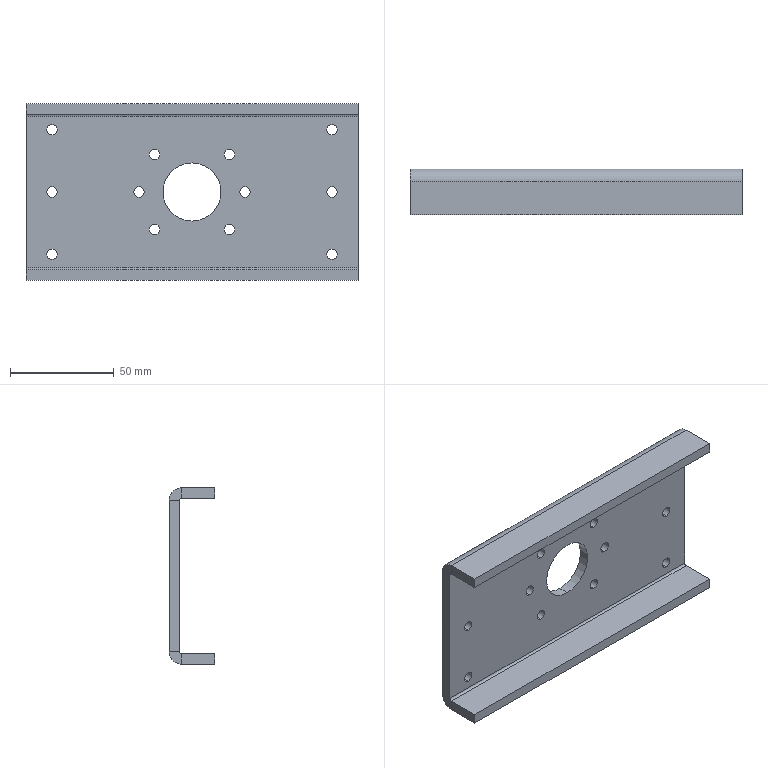Part | SolidWorks | features HoleWzd 2, CirPattern 1, EdgeFlange 1, FlatPattern 1, SMBaseFlange 1, SheetMetal 1 | 1 solid | 48 faces | box 160 x 22 x 85 mm | volume 88540 mm3 | cylinder 30 | plane 18 | commonest cylinder face diameters 5 x24 2 x2 12 x2 28 x2
STEP:
#1=CARTESIAN_POINT('',(18.031,-5.,-20.531));
#2=VERTEX_POINT('',#1);
#3=CARTESIAN_POINT('',(18.031,-5.,-15.531));
#4=VERTEX_POINT('',#3);
#5=CARTESIAN_POINT('',(18.031,-5.,-18.031));
#6=DIRECTION('',(0.,1.,0.));
#7=DIRECTION('',(0.,0.,1.));
#8=AXIS2_PLACEMENT_3D('',#5,#6,#7);
#9=CIRCLE('',#8,2.5);
#10=EDGE_CURVE('',#2,#4,#9,.T.);
#11=ORIENTED_EDGE('',*,*,#10,.F.);
#12=CARTESIAN_POINT('',(18.031,0.,-20.531));
#13=VERTEX_POINT('',#12);
#14=CARTESIAN_POINT('',(18.031,0.,-20.531));
#15=DIRECTION('',(0.,1.,0.));
#16=VECTOR('',#15,1000.);
#17=LINE('',#14,#16);
#18=EDGE_CURVE('',#2,#13,#17,.T.);
#19=ORIENTED_EDGE('',*,*,#18,.T.);
#20=CARTESIAN_POINT('',(18.031,0.,-15.531));
#21=VERTEX_POINT('',#20);
#22=CARTESIAN_POINT('',(18.031,0.,-18.031));
#23=DIRECTION('',(0.,1.,0.));
#24=DIRECTION('',(0.,0.,1.));
#25=AXIS2_PLACEMENT_3D('',#22,#23,#24);
#26=CIRCLE('',#25,2.5);
#27=EDGE_CURVE('',#13,#21,#26,.T.);
#28=ORIENTED_EDGE('',*,*,#27,.T.);
#29=CARTESIAN_POINT('',(18.031,0.,-15.531));
#30=DIRECTION('',(0.,1.,0.));
#31=VECTOR('',#30,1000.);
#32=LINE('',#29,#31);
#33=EDGE_CURVE('',#4,#21,#32,.T.);
#34=ORIENTED_EDGE('',*,*,#33,.F.);
#35=EDGE_LOOP('',(#11,#19,#28,#34));
#36=FACE_OUTER_BOUND('',#35,.T.);
#37=CARTESIAN_POINT('',(18.031,0.,-18.031));
#38=DIRECTION('',(0.,1.,0.));
#39=DIRECTION('',(0.,0.,1.));
#40=AXIS2_PLACEMENT_3D('',#37,#38,#39);
#41=CYLINDRICAL_SURFACE('',#40,2.5);
#42=ADVANCED_FACE('',(#36),#41,.F.);
#43=CARTESIAN_POINT('',(25.5,-5.,-2.5));
#44=VERTEX_POINT('',#43);
#45=CARTESIAN_POINT('',(25.5,-5.,2.5));
#46=VERTEX_POINT('',#45);
#47=CARTESIAN_POINT('',(25.5,-5.,0.));
#48=DIRECTION('',(0.,1.,0.));
#49=DIRECTION('',(0.,0.,1.));
#50=AXIS2_PLACEMENT_3D('',#47,#48,#49);
#51=CIRCLE('',#50,2.5);
#52=EDGE_CURVE('',#44,#46,#51,.T.);
#53=ORIENTED_EDGE('',*,*,#52,.F.);
#54=CARTESIAN_POINT('',(25.5,0.,-2.5));
#55=VERTEX_POINT('',#54);
#56=CARTESIAN_POINT('',(25.5,0.,-2.5));
#57=DIRECTION('',(0.,1.,0.));
#58=VECTOR('',#57,1000.);
#59=LINE('',#56,#58);
#60=EDGE_CURVE('',#44,#55,#59,.T.);
#61=ORIENTED_EDGE('',*,*,#60,.T.);
#62=CARTESIAN_POINT('',(25.5,0.,2.5));
#63=VERTEX_POINT('',#62);
#64=CARTESIAN_POINT('',(25.5,0.,0.));
#65=DIRECTION('',(0.,1.,0.));
#66=DIRECTION('',(0.,0.,1.));
#67=AXIS2_PLACEMENT_3D('',#64,#65,#66);
#68=CIRCLE('',#67,2.5);
#69=EDGE_CURVE('',#55,#63,#68,.T.);
#70=ORIENTED_EDGE('',*,*,#69,.T.);
#71=CARTESIAN_POINT('',(25.5,0.,2.5));
#72=DIRECTION('',(0.,1.,0.));
#73=VECTOR('',#72,1000.);
#74=LINE('',#71,#73);
#75=EDGE_CURVE('',#46,#63,#74,.T.);
#76=ORIENTED_EDGE('',*,*,#75,.F.);
#77=EDGE_LOOP('',(#53,#61,#70,#76));
#78=FACE_OUTER_BOUND('',#77,.T.);
#79=CARTESIAN_POINT('',(25.5,0.,0.));
#80=DIRECTION('',(0.,1.,0.));
#81=DIRECTION('',(0.,0.,1.));
#82=AXIS2_PLACEMENT_3D('',#79,#80,#81);
#83=CYLINDRICAL_SURFACE('',#82,2.5);
#84=ADVANCED_FACE('',(#78),#83,.F.);
#85=CARTESIAN_POINT('',(18.031,-5.,15.531));
#86=VERTEX_POINT('',#85);
#87=CARTESIAN_POINT('',(18.031,-5.,20.531));
#88=VERTEX_POINT('',#87);
#89=CARTESIAN_POINT('',(18.031,-5.,18.031));
#90=DIRECTION('',(0.,1.,0.));
#91=DIRECTION('',(0.,0.,1.));
#92=AXIS2_PLACEMENT_3D('',#89,#90,#91);
#93=CIRCLE('',#92,2.5);
#94=EDGE_CURVE('',#86,#88,#93,.T.);
#95=ORIENTED_EDGE('',*,*,#94,.F.);
#96=CARTESIAN_POINT('',(18.031,0.,15.531));
#97=VERTEX_POINT('',#96);
#98=CARTESIAN_POINT('',(18.031,0.,15.531));
#99=DIRECTION('',(0.,1.,0.));
#100=VECTOR('',#99,1000.);
#101=LINE('',#98,#100);
#102=EDGE_CURVE('',#86,#97,#101,.T.);
#103=ORIENTED_EDGE('',*,*,#102,.T.);
#104=CARTESIAN_POINT('',(18.031,0.,20.531));
#105=VERTEX_POINT('',#104);
#106=CARTESIAN_POINT('',(18.031,0.,18.031));
#107=DIRECTION('',(0.,1.,0.));
#108=DIRECTION('',(0.,0.,1.));
#109=AXIS2_PLACEMENT_3D('',#106,#107,#108);
#110=CIRCLE('',#109,2.5);
#111=EDGE_CURVE('',#97,#105,#110,.T.);
#112=ORIENTED_EDGE('',*,*,#111,.T.);
#113=CARTESIAN_POINT('',(18.031,0.,20.531));
#114=DIRECTION('',(0.,1.,0.));
#115=VECTOR('',#114,1000.);
#116=LINE('',#113,#115);
#117=EDGE_CURVE('',#88,#105,#116,.T.);
#118=ORIENTED_EDGE('',*,*,#117,.F.);
#119=EDGE_LOOP('',(#95,#103,#112,#118));
#120=FACE_OUTER_BOUND('',#119,.T.);
#121=CARTESIAN_POINT('',(18.031,0.,18.031));
#122=DIRECTION('',(0.,1.,0.));
#123=DIRECTION('',(0.,0.,1.));
#124=AXIS2_PLACEMENT_3D('',#121,#122,#123);
#125=CYLINDRICAL_SURFACE('',#124,2.5);
#126=ADVANCED_FACE('',(#120),#125,.F.);
#127=CARTESIAN_POINT('',(-18.031,-5.,15.531));
#128=VERTEX_POINT('',#127);
#129=CARTESIAN_POINT('',(-18.031,-5.,20.531));
#130=VERTEX_POINT('',#129);
#131=CARTESIAN_POINT('',(-18.031,-5.,18.031));
#132=DIRECTION('',(0.,1.,0.));
#133=DIRECTION('',(0.,0.,1.));
#134=AXIS2_PLACEMENT_3D('',#131,#132,#133);
#135=CIRCLE('',#134,2.5);
#136=EDGE_CURVE('',#128,#130,#135,.T.);
#137=ORIENTED_EDGE('',*,*,#136,.F.);
#138=CARTESIAN_POINT('',(-18.031,0.,15.531));
#139=VERTEX_POINT('',#138);
#140=CARTESIAN_POINT('',(-18.031,0.,15.531));
#141=DIRECTION('',(0.,1.,0.));
#142=VECTOR('',#141,1000.);
#143=LINE('',#140,#142);
#144=EDGE_CURVE('',#128,#139,#143,.T.);
#145=ORIENTED_EDGE('',*,*,#144,.T.);
#146=CARTESIAN_POINT('',(-18.031,0.,20.531));
#147=VERTEX_POINT('',#146);
#148=CARTESIAN_POINT('',(-18.031,0.,18.031));
#149=DIRECTION('',(0.,1.,0.));
#150=DIRECTION('',(0.,0.,1.));
#151=AXIS2_PLACEMENT_3D('',#148,#149,#150);
#152=CIRCLE('',#151,2.5);
#153=EDGE_CURVE('',#139,#147,#152,.T.);
#154=ORIENTED_EDGE('',*,*,#153,.T.);
#155=CARTESIAN_POINT('',(-18.031,0.,20.531));
#156=DIRECTION('',(0.,1.,0.));
#157=VECTOR('',#156,1000.);
#158=LINE('',#155,#157);
#159=EDGE_CURVE('',#130,#147,#158,.T.);
#160=ORIENTED_EDGE('',*,*,#159,.F.);
#161=EDGE_LOOP('',(#137,#145,#154,#160));
#162=FACE_OUTER_BOUND('',#161,.T.);
#163=CARTESIAN_POINT('',(-18.031,0.,18.031));
#164=DIRECTION('',(0.,1.,0.));
#165=DIRECTION('',(0.,0.,1.));
#166=AXIS2_PLACEMENT_3D('',#163,#164,#165);
#167=CYLINDRICAL_SURFACE('',#166,2.5);
#168=ADVANCED_FACE('',(#162),#167,.F.);
#169=CARTESIAN_POINT('',(-25.5,-5.,-2.5));
#170=VERTEX_POINT('',#169);
#171=CARTESIAN_POINT('',(-25.5,-5.,2.5));
#172=VERTEX_POINT('',#171);
#173=CARTESIAN_POINT('',(-25.5,-5.,0.));
#174=DIRECTION('',(0.,1.,0.));
#175=DIRECTION('',(0.,0.,1.));
#176=AXIS2_PLACEMENT_3D('',#173,#174,#175);
#177=CIRCLE('',#176,2.5);
#178=EDGE_CURVE('',#170,#172,#177,.T.);
#179=ORIENTED_EDGE('',*,*,#178,.F.);
#180=CARTESIAN_POINT('',(-25.5,0.,-2.5));
#181=VERTEX_POINT('',#180);
#182=CARTESIAN_POINT('',(-25.5,0.,-2.5));
#183=DIRECTION('',(0.,1.,0.));
#184=VECTOR('',#183,1000.);
#185=LINE('',#182,#184);
#186=EDGE_CURVE('',#170,#181,#185,.T.);
#187=ORIENTED_EDGE('',*,*,#186,.T.);
#188=CARTESIAN_POINT('',(-25.5,0.,2.5));
#189=VERTEX_POINT('',#188);
#190=CARTESIAN_POINT('',(-25.5,0.,0.));
#191=DIRECTION('',(0.,1.,0.));
#192=DIRECTION('',(0.,0.,1.));
#193=AXIS2_PLACEMENT_3D('',#190,#191,#192);
#194=CIRCLE('',#193,2.5);
#195=EDGE_CURVE('',#181,#189,#194,.T.);
#196=ORIENTED_EDGE('',*,*,#195,.T.);
#197=CARTESIAN_POINT('',(-25.5,0.,2.5));
#198=DIRECTION('',(0.,1.,0.));
#199=VECTOR('',#198,1000.);
#200=LINE('',#197,#199);
#201=EDGE_CURVE('',#172,#189,#200,.T.);
#202=ORIENTED_EDGE('',*,*,#201,.F.);
#203=EDGE_LOOP('',(#179,#187,#196,#202));
#204=FACE_OUTER_BOUND('',#203,.T.);
#205=CARTESIAN_POINT('',(-25.5,0.,0.));
#206=DIRECTION('',(0.,1.,0.));
#207=DIRECTION('',(0.,0.,1.));
#208=AXIS2_PLACEMENT_3D('',#205,#206,#207);
#209=CYLINDRICAL_SURFACE('',#208,2.5);
#210=ADVANCED_FACE('',(#204),#209,.F.);
#211=CARTESIAN_POINT('',(-18.031,-5.,-20.531));
#212=VERTEX_POINT('',#211);
#213=CARTESIAN_POINT('',(-18.031,-5.,-15.531));
#214=VERTEX_POINT('',#213);
#215=CARTESIAN_POINT('',(-18.031,-5.,-18.031));
#216=DIRECTION('',(0.,1.,0.));
#217=DIRECTION('',(0.,0.,1.));
#218=AXIS2_PLACEMENT_3D('',#215,#216,#217);
#219=CIRCLE('',#218,2.5);
#220=EDGE_CURVE('',#212,#214,#219,.T.);
#221=ORIENTED_EDGE('',*,*,#220,.F.);
#222=CARTESIAN_POINT('',(-18.031,0.,-20.531));
#223=VERTEX_POINT('',#222);
#224=CARTESIAN_POINT('',(-18.031,0.,-20.531));
#225=DIRECTION('',(0.,1.,0.));
#226=VECTOR('',#225,1000.);
#227=LINE('',#224,#226);
#228=EDGE_CURVE('',#212,#223,#227,.T.);
#229=ORIENTED_EDGE('',*,*,#228,.T.);
#230=CARTESIAN_POINT('',(-18.031,0.,-15.531));
#231=VERTEX_POINT('',#230);
#232=CARTESIAN_POINT('',(-18.031,0.,-18.031));
#233=DIRECTION('',(0.,1.,0.));
#234=DIRECTION('',(0.,0.,1.));
#235=AXIS2_PLACEMENT_3D('',#232,#233,#234);
#236=CIRCLE('',#235,2.5);
#237=EDGE_CURVE('',#223,#231,#236,.T.);
#238=ORIENTED_EDGE('',*,*,#237,.T.);
#239=CARTESIAN_POINT('',(-18.031,0.,-15.531));
#240=DIRECTION('',(0.,1.,0.));
#241=VECTOR('',#240,1000.);
#242=LINE('',#239,#241);
#243=EDGE_CURVE('',#214,#231,#242,.T.);
#244=ORIENTED_EDGE('',*,*,#243,.F.);
#245=EDGE_LOOP('',(#221,#229,#238,#244));
#246=FACE_OUTER_BOUND('',#245,.T.);
#247=CARTESIAN_POINT('',(-18.031,0.,-18.031));
#248=DIRECTION('',(0.,1.,0.));
#249=DIRECTION('',(0.,0.,1.));
#250=AXIS2_PLACEMENT_3D('',#247,#248,#249);
#251=CYLINDRICAL_SURFACE('',#250,2.5);
#252=ADVANCED_FACE('',(#246),#251,.F.);
#253=CARTESIAN_POINT('',(-67.5,-5.,-2.5));
#254=VERTEX_POINT('',#253);
#255=CARTESIAN_POINT('',(-67.5,-5.,2.5));
#256=VERTEX_POINT('',#255);
#257=CARTESIAN_POINT('',(-67.5,-5.,0.));
#258=DIRECTION('',(0.,1.,0.));
#259=DIRECTION('',(0.,0.,1.));
#260=AXIS2_PLACEMENT_3D('',#257,#258,#259);
#261=CIRCLE('',#260,2.5);
#262=EDGE_CURVE('',#254,#256,#261,.T.);
#263=ORIENTED_EDGE('',*,*,#262,.F.);
#264=CARTESIAN_POINT('',(-67.5,0.,-2.5));
#265=VERTEX_POINT('',#264);
#266=CARTESIAN_POINT('',(-67.5,0.,-2.5));
#267=DIRECTION('',(0.,1.,0.));
#268=VECTOR('',#267,1000.);
#269=LINE('',#266,#268);
#270=EDGE_CURVE('',#254,#265,#269,.T.);
#271=ORIENTED_EDGE('',*,*,#270,.T.);
#272=CARTESIAN_POINT('',(-67.5,0.,2.5));
#273=VERTEX_POINT('',#272);
#274=CARTESIAN_POINT('',(-67.5,0.,0.));
#275=DIRECTION('',(0.,1.,0.));
#276=DIRECTION('',(0.,0.,1.));
#277=AXIS2_PLACEMENT_3D('',#274,#275,#276);
#278=CIRCLE('',#277,2.5);
#279=EDGE_CURVE('',#265,#273,#278,.T.);
#280=ORIENTED_EDGE('',*,*,#279,.T.);
#281=CARTESIAN_POINT('',(-67.5,0.,2.5));
#282=DIRECTION('',(0.,1.,0.));
#283=VECTOR('',#282,1000.);
#284=LINE('',#281,#283);
#285=EDGE_CURVE('',#256,#273,#284,.T.);
#286=ORIENTED_EDGE('',*,*,#285,.F.);
#287=EDGE_LOOP('',(#263,#271,#280,#286));
#288=FACE_OUTER_BOUND('',#287,.T.);
#289=CARTESIAN_POINT('',(-67.5,0.,0.));
#290=DIRECTION('',(0.,1.,0.));
#291=DIRECTION('',(0.,0.,1.));
#292=AXIS2_PLACEMENT_3D('',#289,#290,#291);
#293=CYLINDRICAL_SURFACE('',#292,2.5);
#294=ADVANCED_FACE('',(#288),#293,.F.);
#295=CARTESIAN_POINT('',(-67.5,-5.,-32.5));
#296=VERTEX_POINT('',#295);
#297=CARTESIAN_POINT('',(-67.5,-5.,-27.5));
#298=VERTEX_POINT('',#297);
#299=CARTESIAN_POINT('',(-67.5,-5.,-30.));
#300=DIRECTION('',(0.,1.,0.));
#301=DIRECTION('',(0.,0.,1.));
#302=AXIS2_PLACEMENT_3D('',#299,#300,#301);
#303=CIRCLE('',#302,2.5);
#304=EDGE_CURVE('',#296,#298,#303,.T.);
#305=ORIENTED_EDGE('',*,*,#304,.F.);
#306=CARTESIAN_POINT('',(-67.5,0.,-32.5));
#307=VERTEX_POINT('',#306);
#308=CARTESIAN_POINT('',(-67.5,0.,-32.5));
#309=DIRECTION('',(0.,1.,0.));
#310=VECTOR('',#309,1000.);
#311=LINE('',#308,#310);
#312=EDGE_CURVE('',#296,#307,#311,.T.);
#313=ORIENTED_EDGE('',*,*,#312,.T.);
#314=CARTESIAN_POINT('',(-67.5,0.,-27.5));
#315=VERTEX_POINT('',#314);
#316=CARTESIAN_POINT('',(-67.5,0.,-30.));
#317=DIRECTION('',(0.,1.,0.));
#318=DIRECTION('',(0.,0.,1.));
#319=AXIS2_PLACEMENT_3D('',#316,#317,#318);
#320=CIRCLE('',#319,2.5);
#321=EDGE_CURVE('',#307,#315,#320,.T.);
#322=ORIENTED_EDGE('',*,*,#321,.T.);
#323=CARTESIAN_POINT('',(-67.5,0.,-27.5));
#324=DIRECTION('',(0.,1.,0.));
#325=VECTOR('',#324,1000.);
#326=LINE('',#323,#325);
#327=EDGE_CURVE('',#298,#315,#326,.T.);
#328=ORIENTED_EDGE('',*,*,#327,.F.);
#329=EDGE_LOOP('',(#305,#313,#322,#328));
#330=FACE_OUTER_BOUND('',#329,.T.);
#331=CARTESIAN_POINT('',(-67.5,0.,-30.));
#332=DIRECTION('',(0.,1.,0.));
#333=DIRECTION('',(0.,0.,1.));
#334=AXIS2_PLACEMENT_3D('',#331,#332,#333);
#335=CYLINDRICAL_SURFACE('',#334,2.5);
#336=ADVANCED_FACE('',(#330),#335,.F.);
#337=CARTESIAN_POINT('',(-67.5,-5.,27.5));
#338=VERTEX_POINT('',#337);
#339=CARTESIAN_POINT('',(-67.5,-5.,32.5));
#340=VERTEX_POINT('',#339);
#341=CARTESIAN_POINT('',(-67.5,-5.,30.));
#342=DIRECTION('',(0.,1.,0.));
#343=DIRECTION('',(0.,0.,1.));
#344=AXIS2_PLACEMENT_3D('',#341,#342,#343);
#345=CIRCLE('',#344,2.5);
#346=EDGE_CURVE('',#338,#340,#345,.T.);
#347=ORIENTED_EDGE('',*,*,#346,.F.);
#348=CARTESIAN_POINT('',(-67.5,0.,27.5));
#349=VERTEX_POINT('',#348);
#350=CARTESIAN_POINT('',(-67.5,0.,27.5));
#351=DIRECTION('',(0.,1.,0.));
#352=VECTOR('',#351,1000.);
#353=LINE('',#350,#352);
#354=EDGE_CURVE('',#338,#349,#353,.T.);
#355=ORIENTED_EDGE('',*,*,#354,.T.);
#356=CARTESIAN_POINT('',(-67.5,0.,32.5));
#357=VERTEX_POINT('',#356);
#358=CARTESIAN_POINT('',(-67.5,0.,30.));
#359=DIRECTION('',(0.,1.,0.));
#360=DIRECTION('',(0.,0.,1.));
#361=AXIS2_PLACEMENT_3D('',#358,#359,#360);
#362=CIRCLE('',#361,2.5);
#363=EDGE_CURVE('',#349,#357,#362,.T.);
#364=ORIENTED_EDGE('',*,*,#363,.T.);
#365=CARTESIAN_POINT('',(-67.5,0.,32.5));
#366=DIRECTION('',(0.,1.,0.));
#367=VECTOR('',#366,1000.);
#368=LINE('',#365,#367);
#369=EDGE_CURVE('',#340,#357,#368,.T.);
#370=ORIENTED_EDGE('',*,*,#369,.F.);
#371=EDGE_LOOP('',(#347,#355,#364,#370));
#372=FACE_OUTER_BOUND('',#371,.T.);
#373=CARTESIAN_POINT('',(-67.5,0.,30.));
#374=DIRECTION('',(0.,1.,0.));
#375=DIRECTION('',(0.,0.,1.));
#376=AXIS2_PLACEMENT_3D('',#373,#374,#375);
#377=CYLINDRICAL_SURFACE('',#376,2.5);
#378=ADVANCED_FACE('',(#372),#377,.F.);
#379=CARTESIAN_POINT('',(67.5,-5.,27.5));
#380=VERTEX_POINT('',#379);
#381=CARTESIAN_POINT('',(67.5,-5.,32.5));
#382=VERTEX_POINT('',#381);
#383=CARTESIAN_POINT('',(67.5,-5.,30.));
#384=DIRECTION('',(0.,1.,0.));
#385=DIRECTION('',(0.,0.,1.));
#386=AXIS2_PLACEMENT_3D('',#383,#384,#385);
#387=CIRCLE('',#386,2.5);
#388=EDGE_CURVE('',#380,#382,#387,.T.);
#389=ORIENTED_EDGE('',*,*,#388,.F.);
#390=CARTESIAN_POINT('',(67.5,0.,27.5));
#391=VERTEX_POINT('',#390);
#392=CARTESIAN_POINT('',(67.5,0.,27.5));
#393=DIRECTION('',(0.,1.,0.));
#394=VECTOR('',#393,1000.);
#395=LINE('',#392,#394);
#396=EDGE_CURVE('',#380,#391,#395,.T.);
#397=ORIENTED_EDGE('',*,*,#396,.T.);
#398=CARTESIAN_POINT('',(67.5,0.,32.5));
#399=VERTEX_POINT('',#398);
#400=CARTESIAN_POINT('',(67.5,0.,30.));
#401=DIRECTION('',(0.,1.,0.));
#402=DIRECTION('',(0.,0.,1.));
#403=AXIS2_PLACEMENT_3D('',#400,#401,#402);
#404=CIRCLE('',#403,2.5);
#405=EDGE_CURVE('',#391,#399,#404,.T.);
#406=ORIENTED_EDGE('',*,*,#405,.T.);
#407=CARTESIAN_POINT('',(67.5,0.,32.5));
#408=DIRECTION('',(0.,1.,0.));
#409=VECTOR('',#408,1000.);
#410=LINE('',#407,#409);
#411=EDGE_CURVE('',#382,#399,#410,.T.);
#412=ORIENTED_EDGE('',*,*,#411,.F.);
#413=EDGE_LOOP('',(#389,#397,#406,#412));
#414=FACE_OUTER_BOUND('',#413,.T.);
#415=CARTESIAN_POINT('',(67.5,0.,30.));
#416=DIRECTION('',(0.,1.,0.));
#417=DIRECTION('',(0.,0.,1.));
#418=AXIS2_PLACEMENT_3D('',#415,#416,#417);
#419=CYLINDRICAL_SURFACE('',#418,2.5);
#420=ADVANCED_FACE('',(#414),#419,.F.);
#421=CARTESIAN_POINT('',(67.5,-5.,-32.5));
#422=VERTEX_POINT('',#421);
#423=CARTESIAN_POINT('',(67.5,-5.,-27.5));
#424=VERTEX_POINT('',#423);
#425=CARTESIAN_POINT('',(67.5,-5.,-30.));
#426=DIRECTION('',(0.,1.,0.));
#427=DIRECTION('',(0.,0.,1.));
#428=AXIS2_PLACEMENT_3D('',#425,#426,#427);
#429=CIRCLE('',#428,2.5);
#430=EDGE_CURVE('',#422,#424,#429,.T.);
#431=ORIENTED_EDGE('',*,*,#430,.F.);
#432=CARTESIAN_POINT('',(67.5,0.,-32.5));
#433=VERTEX_POINT('',#432);
#434=CARTESIAN_POINT('',(67.5,0.,-32.5));
#435=DIRECTION('',(0.,1.,0.));
#436=VECTOR('',#435,1000.);
#437=LINE('',#434,#436);
#438=EDGE_CURVE('',#422,#433,#437,.T.);
#439=ORIENTED_EDGE('',*,*,#438,.T.);
#440=CARTESIAN_POINT('',(67.5,0.,-27.5));
#441=VERTEX_POINT('',#440);
#442=CARTESIAN_POINT('',(67.5,0.,-30.));
#443=DIRECTION('',(0.,1.,0.));
#444=DIRECTION('',(0.,0.,1.));
#445=AXIS2_PLACEMENT_3D('',#442,#443,#444);
#446=CIRCLE('',#445,2.5);
#447=EDGE_CURVE('',#433,#441,#446,.T.);
#448=ORIENTED_EDGE('',*,*,#447,.T.);
#449=CARTESIAN_POINT('',(67.5,0.,-27.5));
#450=DIRECTION('',(0.,1.,0.));
#451=VECTOR('',#450,1000.);
#452=LINE('',#449,#451);
#453=EDGE_CURVE('',#424,#441,#452,.T.);
#454=ORIENTED_EDGE('',*,*,#453,.F.);
#455=EDGE_LOOP('',(#431,#439,#448,#454));
#456=FACE_OUTER_BOUND('',#455,.T.);
#457=CARTESIAN_POINT('',(67.5,0.,-30.));
#458=DIRECTION('',(0.,1.,0.));
#459=DIRECTION('',(0.,0.,1.));
#460=AXIS2_PLACEMENT_3D('',#457,#458,#459);
#461=CYLINDRICAL_SURFACE('',#460,2.5);
#462=ADVANCED_FACE('',(#456),#461,.F.);
#463=CARTESIAN_POINT('',(67.5,-5.,-2.5));
#464=VERTEX_POINT('',#463);
#465=CARTESIAN_POINT('',(67.5,-5.,2.5));
#466=VERTEX_POINT('',#465);
#467=CARTESIAN_POINT('',(67.5,-5.,0.));
#468=DIRECTION('',(0.,1.,0.));
#469=DIRECTION('',(0.,0.,1.));
#470=AXIS2_PLACEMENT_3D('',#467,#468,#469);
#471=CIRCLE('',#470,2.5);
#472=EDGE_CURVE('',#464,#466,#471,.T.);
#473=ORIENTED_EDGE('',*,*,#472,.F.);
#474=CARTESIAN_POINT('',(67.5,0.,-2.5));
#475=VERTEX_POINT('',#474);
#476=CARTESIAN_POINT('',(67.5,0.,-2.5));
#477=DIRECTION('',(0.,1.,0.));
#478=VECTOR('',#477,1000.);
#479=LINE('',#476,#478);
#480=EDGE_CURVE('',#464,#475,#479,.T.);
#481=ORIENTED_EDGE('',*,*,#480,.T.);
#482=CARTESIAN_POINT('',(67.5,0.,2.5));
#483=VERTEX_POINT('',#482);
#484=CARTESIAN_POINT('',(67.5,0.,0.));
#485=DIRECTION('',(0.,1.,0.));
#486=DIRECTION('',(0.,0.,1.));
#487=AXIS2_PLACEMENT_3D('',#484,#485,#486);
#488=CIRCLE('',#487,2.5);
#489=EDGE_CURVE('',#475,#483,#488,.T.);
#490=ORIENTED_EDGE('',*,*,#489,.T.);
#491=CARTESIAN_POINT('',(67.5,0.,2.5));
#492=DIRECTION('',(0.,1.,0.));
#493=VECTOR('',#492,1000.);
#494=LINE('',#491,#493);
#495=EDGE_CURVE('',#466,#483,#494,.T.);
#496=ORIENTED_EDGE('',*,*,#495,.F.);
#497=EDGE_LOOP('',(#473,#481,#490,#496));
#498=FACE_OUTER_BOUND('',#497,.T.);
#499=CARTESIAN_POINT('',(67.5,0.,0.));
#500=DIRECTION('',(0.,1.,0.));
#501=DIRECTION('',(0.,0.,1.));
#502=AXIS2_PLACEMENT_3D('',#499,#500,#501);
#503=CYLINDRICAL_SURFACE('',#502,2.5);
#504=ADVANCED_FACE('',(#498),#503,.F.);
#505=CARTESIAN_POINT('',(0.,-5.,-14.));
#506=VERTEX_POINT('',#505);
#507=CARTESIAN_POINT('',(0.,-5.,14.));
#508=VERTEX_POINT('',#507);
#509=CARTESIAN_POINT('',(0.,-5.,0.));
#510=DIRECTION('',(0.,1.,0.));
#511=DIRECTION('',(0.,0.,1.));
#512=AXIS2_PLACEMENT_3D('',#509,#510,#511);
#513=CIRCLE('',#512,14.);
#514=EDGE_CURVE('',#506,#508,#513,.T.);
#515=ORIENTED_EDGE('',*,*,#514,.F.);
#516=CARTESIAN_POINT('',(0.,0.,-14.));
#517=VERTEX_POINT('',#516);
#518=CARTESIAN_POINT('',(0.,-5.,-14.));
#519=DIRECTION('',(0.,1.,0.));
#520=VECTOR('',#519,1000.);
#521=LINE('',#518,#520);
#522=EDGE_CURVE('',#506,#517,#521,.T.);
#523=ORIENTED_EDGE('',*,*,#522,.T.);
#524=CARTESIAN_POINT('',(0.,0.,14.));
#525=VERTEX_POINT('',#524);
#526=CARTESIAN_POINT('',(0.,0.,0.));
#527=DIRECTION('',(0.,1.,0.));
#528=DIRECTION('',(0.,0.,1.));
#529=AXIS2_PLACEMENT_3D('',#526,#527,#528);
#530=CIRCLE('',#529,14.);
#531=EDGE_CURVE('',#517,#525,#530,.T.);
#532=ORIENTED_EDGE('',*,*,#531,.T.);
#533=CARTESIAN_POINT('',(0.,-5.,14.));
#534=DIRECTION('',(0.,1.,0.));
#535=VECTOR('',#534,1000.);
#536=LINE('',#533,#535);
#537=EDGE_CURVE('',#508,#525,#536,.T.);
#538=ORIENTED_EDGE('',*,*,#537,.F.);
#539=EDGE_LOOP('',(#515,#523,#532,#538));
#540=FACE_OUTER_BOUND('',#539,.T.);
#541=CARTESIAN_POINT('',(0.,-5.,0.));
#542=DIRECTION('',(0.,1.,0.));
#543=DIRECTION('',(0.,0.,1.));
#544=AXIS2_PLACEMENT_3D('',#541,#542,#543);
#545=CYLINDRICAL_SURFACE('',#544,14.);
#546=ADVANCED_FACE('',(#540),#545,.F.);
#547=CARTESIAN_POINT('',(18.031,-5.,-18.031));
#548=DIRECTION('',(0.,1.,0.));
#549=DIRECTION('',(0.,0.,1.));
#550=AXIS2_PLACEMENT_3D('',#547,#548,#549);
#551=CIRCLE('',#550,2.5);
#552=EDGE_CURVE('',#4,#2,#551,.T.);
#553=ORIENTED_EDGE('',*,*,#552,.T.);
#554=ORIENTED_EDGE('',*,*,#10,.T.);
#555=EDGE_LOOP('',(#553,#554));
#556=FACE_BOUND('',#555,.T.);
#557=CARTESIAN_POINT('',(25.5,-5.,0.));
#558=DIRECTION('',(0.,1.,0.));
#559=DIRECTION('',(0.,0.,1.));
#560=AXIS2_PLACEMENT_3D('',#557,#558,#559);
#561=CIRCLE('',#560,2.5);
#562=EDGE_CURVE('',#46,#44,#561,.T.);
#563=ORIENTED_EDGE('',*,*,#562,.T.);
#564=ORIENTED_EDGE('',*,*,#52,.T.);
#565=EDGE_LOOP('',(#563,#564));
#566=FACE_BOUND('',#565,.T.);
#567=CARTESIAN_POINT('',(18.031,-5.,18.031));
#568=DIRECTION('',(0.,1.,0.));
#569=DIRECTION('',(0.,0.,1.));
#570=AXIS2_PLACEMENT_3D('',#567,#568,#569);
#571=CIRCLE('',#570,2.5);
#572=EDGE_CURVE('',#88,#86,#571,.T.);
#573=ORIENTED_EDGE('',*,*,#572,.T.);
#574=ORIENTED_EDGE('',*,*,#94,.T.);
#575=EDGE_LOOP('',(#573,#574));
#576=FACE_BOUND('',#575,.T.);
#577=CARTESIAN_POINT('',(-18.031,-5.,18.031));
#578=DIRECTION('',(0.,1.,0.));
#579=DIRECTION('',(0.,0.,1.));
#580=AXIS2_PLACEMENT_3D('',#577,#578,#579);
#581=CIRCLE('',#580,2.5);
#582=EDGE_CURVE('',#130,#128,#581,.T.);
#583=ORIENTED_EDGE('',*,*,#582,.T.);
#584=ORIENTED_EDGE('',*,*,#136,.T.);
#585=EDGE_LOOP('',(#583,#584));
#586=FACE_BOUND('',#585,.T.);
#587=CARTESIAN_POINT('',(-25.5,-5.,0.));
#588=DIRECTION('',(0.,1.,0.));
#589=DIRECTION('',(0.,0.,1.));
#590=AXIS2_PLACEMENT_3D('',#587,#588,#589);
#591=CIRCLE('',#590,2.5);
#592=EDGE_CURVE('',#172,#170,#591,.T.);
#593=ORIENTED_EDGE('',*,*,#592,.T.);
#594=ORIENTED_EDGE('',*,*,#178,.T.);
#595=EDGE_LOOP('',(#593,#594));
#596=FACE_BOUND('',#595,.T.);
#597=CARTESIAN_POINT('',(-18.031,-5.,-18.031));
#598=DIRECTION('',(0.,1.,0.));
#599=DIRECTION('',(0.,0.,1.));
#600=AXIS2_PLACEMENT_3D('',#597,#598,#599);
#601=CIRCLE('',#600,2.5);
#602=EDGE_CURVE('',#214,#212,#601,.T.);
#603=ORIENTED_EDGE('',*,*,#602,.T.);
#604=ORIENTED_EDGE('',*,*,#220,.T.);
#605=EDGE_LOOP('',(#603,#604));
#606=FACE_BOUND('',#605,.T.);
#607=CARTESIAN_POINT('',(-67.5,-5.,0.));
#608=DIRECTION('',(0.,1.,0.));
#609=DIRECTION('',(0.,0.,1.));
#610=AXIS2_PLACEMENT_3D('',#607,#608,#609);
#611=CIRCLE('',#610,2.5);
#612=EDGE_CURVE('',#256,#254,#611,.T.);
#613=ORIENTED_EDGE('',*,*,#612,.T.);
#614=ORIENTED_EDGE('',*,*,#262,.T.);
#615=EDGE_LOOP('',(#613,#614));
#616=FACE_BOUND('',#615,.T.);
#617=CARTESIAN_POINT('',(-67.5,-5.,-30.));
#618=DIRECTION('',(0.,1.,0.));
#619=DIRECTION('',(0.,0.,1.));
#620=AXIS2_PLACEMENT_3D('',#617,#618,#619);
#621=CIRCLE('',#620,2.5);
#622=EDGE_CURVE('',#298,#296,#621,.T.);
#623=ORIENTED_EDGE('',*,*,#622,.T.);
#624=ORIENTED_EDGE('',*,*,#304,.T.);
#625=EDGE_LOOP('',(#623,#624));
#626=FACE_BOUND('',#625,.T.);
#627=CARTESIAN_POINT('',(-67.5,-5.,30.));
#628=DIRECTION('',(0.,1.,0.));
#629=DIRECTION('',(0.,0.,1.));
#630=AXIS2_PLACEMENT_3D('',#627,#628,#629);
#631=CIRCLE('',#630,2.5);
#632=EDGE_CURVE('',#340,#338,#631,.T.);
#633=ORIENTED_EDGE('',*,*,#632,.T.);
#634=ORIENTED_EDGE('',*,*,#346,.T.);
#635=EDGE_LOOP('',(#633,#634));
#636=FACE_BOUND('',#635,.T.);
#637=CARTESIAN_POINT('',(67.5,-5.,30.));
#638=DIRECTION('',(0.,1.,0.));
#639=DIRECTION('',(0.,0.,1.));
#640=AXIS2_PLACEMENT_3D('',#637,#638,#639);
#641=CIRCLE('',#640,2.5);
#642=EDGE_CURVE('',#382,#380,#641,.T.);
#643=ORIENTED_EDGE('',*,*,#642,.T.);
#644=ORIENTED_EDGE('',*,*,#388,.T.);
#645=EDGE_LOOP('',(#643,#644));
#646=FACE_BOUND('',#645,.T.);
#647=CARTESIAN_POINT('',(67.5,-5.,-30.));
#648=DIRECTION('',(0.,1.,0.));
#649=DIRECTION('',(0.,0.,1.));
#650=AXIS2_PLACEMENT_3D('',#647,#648,#649);
#651=CIRCLE('',#650,2.5);
#652=EDGE_CURVE('',#424,#422,#651,.T.);
#653=ORIENTED_EDGE('',*,*,#652,.T.);
#654=ORIENTED_EDGE('',*,*,#430,.T.);
#655=EDGE_LOOP('',(#653,#654));
#656=FACE_BOUND('',#655,.T.);
#657=CARTESIAN_POINT('',(67.5,-5.,0.));
#658=DIRECTION('',(0.,1.,0.));
#659=DIRECTION('',(0.,0.,1.));
#660=AXIS2_PLACEMENT_3D('',#657,#658,#659);
#661=CIRCLE('',#660,2.5);
#662=EDGE_CURVE('',#466,#464,#661,.T.);
#663=ORIENTED_EDGE('',*,*,#662,.T.);
#664=ORIENTED_EDGE('',*,*,#472,.T.);
#665=EDGE_LOOP('',(#663,#664));
#666=FACE_BOUND('',#665,.T.);
#667=CARTESIAN_POINT('',(0.,-5.,0.));
#668=DIRECTION('',(0.,1.,0.));
#669=DIRECTION('',(0.,0.,1.));
#670=AXIS2_PLACEMENT_3D('',#667,#668,#669);
#671=CIRCLE('',#670,14.);
#672=EDGE_CURVE('',#508,#506,#671,.T.);
#673=ORIENTED_EDGE('',*,*,#672,.T.);
#674=ORIENTED_EDGE('',*,*,#514,.T.);
#675=EDGE_LOOP('',(#673,#674));
#676=FACE_BOUND('',#675,.T.);
#677=CARTESIAN_POINT('',(-80.,-5.,36.5));
#678=VERTEX_POINT('',#677);
#679=CARTESIAN_POINT('',(80.,-5.,36.5));
#680=VERTEX_POINT('',#679);
#681=CARTESIAN_POINT('',(-80.,-5.,36.5));
#682=DIRECTION('',(1.,0.,0.));
#683=VECTOR('',#682,1000.);
#684=LINE('',#681,#683);
#685=EDGE_CURVE('',#678,#680,#684,.T.);
#686=ORIENTED_EDGE('',*,*,#685,.F.);
#687=CARTESIAN_POINT('',(-80.,-5.,-36.5));
#688=VERTEX_POINT('',#687);
#689=CARTESIAN_POINT('',(-80.,-5.,-42.5));
#690=DIRECTION('',(0.,0.,1.));
#691=VECTOR('',#690,1000.);
#692=LINE('',#689,#691);
#693=EDGE_CURVE('',#688,#678,#692,.T.);
#694=ORIENTED_EDGE('',*,*,#693,.F.);
#695=CARTESIAN_POINT('',(80.,-5.,-36.5));
#696=VERTEX_POINT('',#695);
#697=CARTESIAN_POINT('',(80.,-5.,-36.5));
#698=DIRECTION('',(-1.,0.,0.));
#699=VECTOR('',#698,1000.);
#700=LINE('',#697,#699);
#701=EDGE_CURVE('',#696,#688,#700,.T.);
#702=ORIENTED_EDGE('',*,*,#701,.F.);
#703=CARTESIAN_POINT('',(80.,-5.,42.5));
#704=DIRECTION('',(0.,0.,-1.));
#705=VECTOR('',#704,1000.);
#706=LINE('',#703,#705);
#707=EDGE_CURVE('',#680,#696,#706,.T.);
#708=ORIENTED_EDGE('',*,*,#707,.F.);
#709=EDGE_LOOP('',(#686,#694,#702,#708));
#710=FACE_OUTER_BOUND('',#709,.T.);
#711=CARTESIAN_POINT('',(0.,-5.,0.));
#712=DIRECTION('',(0.,1.,0.));
#713=DIRECTION('',(0.,0.,1.));
#714=AXIS2_PLACEMENT_3D('',#711,#712,#713);
#715=PLANE('',#714);
#716=ADVANCED_FACE('',(#556,#566,#576,#586,#596,#606,#616,#626,#636,#646,#656,#666,#676,#710),#715,.F.);
#717=CARTESIAN_POINT('',(18.031,0.,-18.031));
#718=DIRECTION('',(0.,1.,0.));
#719=DIRECTION('',(0.,0.,1.));
#720=AXIS2_PLACEMENT_3D('',#717,#718,#719);
#721=CIRCLE('',#720,2.5);
#722=EDGE_CURVE('',#21,#13,#721,.T.);
#723=ORIENTED_EDGE('',*,*,#722,.F.);
#724=ORIENTED_EDGE('',*,*,#27,.F.);
#725=EDGE_LOOP('',(#723,#724));
#726=FACE_BOUND('',#725,.T.);
#727=CARTESIAN_POINT('',(25.5,0.,0.));
#728=DIRECTION('',(0.,1.,0.));
#729=DIRECTION('',(0.,0.,1.));
#730=AXIS2_PLACEMENT_3D('',#727,#728,#729);
#731=CIRCLE('',#730,2.5);
#732=EDGE_CURVE('',#63,#55,#731,.T.);
#733=ORIENTED_EDGE('',*,*,#732,.F.);
#734=ORIENTED_EDGE('',*,*,#69,.F.);
#735=EDGE_LOOP('',(#733,#734));
#736=FACE_BOUND('',#735,.T.);
#737=CARTESIAN_POINT('',(18.031,0.,18.031));
#738=DIRECTION('',(0.,1.,0.));
#739=DIRECTION('',(0.,0.,1.));
#740=AXIS2_PLACEMENT_3D('',#737,#738,#739);
#741=CIRCLE('',#740,2.5);
#742=EDGE_CURVE('',#105,#97,#741,.T.);
#743=ORIENTED_EDGE('',*,*,#742,.F.);
#744=ORIENTED_EDGE('',*,*,#111,.F.);
#745=EDGE_LOOP('',(#743,#744));
#746=FACE_BOUND('',#745,.T.);
#747=CARTESIAN_POINT('',(-18.031,0.,18.031));
#748=DIRECTION('',(0.,1.,0.));
#749=DIRECTION('',(0.,0.,1.));
#750=AXIS2_PLACEMENT_3D('',#747,#748,#749);
#751=CIRCLE('',#750,2.5);
#752=EDGE_CURVE('',#147,#139,#751,.T.);
#753=ORIENTED_EDGE('',*,*,#752,.F.);
#754=ORIENTED_EDGE('',*,*,#153,.F.);
#755=EDGE_LOOP('',(#753,#754));
#756=FACE_BOUND('',#755,.T.);
#757=CARTESIAN_POINT('',(-25.5,0.,0.));
#758=DIRECTION('',(0.,1.,0.));
#759=DIRECTION('',(0.,0.,1.));
#760=AXIS2_PLACEMENT_3D('',#757,#758,#759);
#761=CIRCLE('',#760,2.5);
#762=EDGE_CURVE('',#189,#181,#761,.T.);
#763=ORIENTED_EDGE('',*,*,#762,.F.);
#764=ORIENTED_EDGE('',*,*,#195,.F.);
#765=EDGE_LOOP('',(#763,#764));
#766=FACE_BOUND('',#765,.T.);
#767=CARTESIAN_POINT('',(-18.031,0.,-18.031));
#768=DIRECTION('',(0.,1.,0.));
#769=DIRECTION('',(0.,0.,1.));
#770=AXIS2_PLACEMENT_3D('',#767,#768,#769);
#771=CIRCLE('',#770,2.5);
#772=EDGE_CURVE('',#231,#223,#771,.T.);
#773=ORIENTED_EDGE('',*,*,#772,.F.);
#774=ORIENTED_EDGE('',*,*,#237,.F.);
#775=EDGE_LOOP('',(#773,#774));
#776=FACE_BOUND('',#775,.T.);
#777=CARTESIAN_POINT('',(-67.5,0.,0.));
#778=DIRECTION('',(0.,1.,0.));
#779=DIRECTION('',(0.,0.,1.));
#780=AXIS2_PLACEMENT_3D('',#777,#778,#779);
#781=CIRCLE('',#780,2.5);
#782=EDGE_CURVE('',#273,#265,#781,.T.);
#783=ORIENTED_EDGE('',*,*,#782,.F.);
#784=ORIENTED_EDGE('',*,*,#279,.F.);
#785=EDGE_LOOP('',(#783,#784));
#786=FACE_BOUND('',#785,.T.);
#787=CARTESIAN_POINT('',(-67.5,0.,-30.));
#788=DIRECTION('',(0.,1.,0.));
#789=DIRECTION('',(0.,0.,1.));
#790=AXIS2_PLACEMENT_3D('',#787,#788,#789);
#791=CIRCLE('',#790,2.5);
#792=EDGE_CURVE('',#315,#307,#791,.T.);
#793=ORIENTED_EDGE('',*,*,#792,.F.);
#794=ORIENTED_EDGE('',*,*,#321,.F.);
#795=EDGE_LOOP('',(#793,#794));
#796=FACE_BOUND('',#795,.T.);
#797=CARTESIAN_POINT('',(-67.5,0.,30.));
#798=DIRECTION('',(0.,1.,0.));
#799=DIRECTION('',(0.,0.,1.));
#800=AXIS2_PLACEMENT_3D('',#797,#798,#799);
#801=CIRCLE('',#800,2.5);
#802=EDGE_CURVE('',#357,#349,#801,.T.);
#803=ORIENTED_EDGE('',*,*,#802,.F.);
#804=ORIENTED_EDGE('',*,*,#363,.F.);
#805=EDGE_LOOP('',(#803,#804));
#806=FACE_BOUND('',#805,.T.);
#807=CARTESIAN_POINT('',(67.5,0.,30.));
#808=DIRECTION('',(0.,1.,0.));
#809=DIRECTION('',(0.,0.,1.));
#810=AXIS2_PLACEMENT_3D('',#807,#808,#809);
#811=CIRCLE('',#810,2.5);
#812=EDGE_CURVE('',#399,#391,#811,.T.);
#813=ORIENTED_EDGE('',*,*,#812,.F.);
#814=ORIENTED_EDGE('',*,*,#405,.F.);
#815=EDGE_LOOP('',(#813,#814));
#816=FACE_BOUND('',#815,.T.);
#817=CARTESIAN_POINT('',(67.5,0.,-30.));
#818=DIRECTION('',(0.,1.,0.));
#819=DIRECTION('',(0.,0.,1.));
#820=AXIS2_PLACEMENT_3D('',#817,#818,#819);
#821=CIRCLE('',#820,2.5);
#822=EDGE_CURVE('',#441,#433,#821,.T.);
#823=ORIENTED_EDGE('',*,*,#822,.F.);
#824=ORIENTED_EDGE('',*,*,#447,.F.);
#825=EDGE_LOOP('',(#823,#824));
#826=FACE_BOUND('',#825,.T.);
#827=CARTESIAN_POINT('',(67.5,0.,0.));
#828=DIRECTION('',(0.,1.,0.));
#829=DIRECTION('',(0.,0.,1.));
#830=AXIS2_PLACEMENT_3D('',#827,#828,#829);
#831=CIRCLE('',#830,2.5);
#832=EDGE_CURVE('',#483,#475,#831,.T.);
#833=ORIENTED_EDGE('',*,*,#832,.F.);
#834=ORIENTED_EDGE('',*,*,#489,.F.);
#835=EDGE_LOOP('',(#833,#834));
#836=FACE_BOUND('',#835,.T.);
#837=CARTESIAN_POINT('',(0.,0.,0.));
#838=DIRECTION('',(0.,1.,0.));
#839=DIRECTION('',(0.,0.,1.));
#840=AXIS2_PLACEMENT_3D('',#837,#838,#839);
#841=CIRCLE('',#840,14.);
#842=EDGE_CURVE('',#525,#517,#841,.T.);
#843=ORIENTED_EDGE('',*,*,#842,.F.);
#844=ORIENTED_EDGE('',*,*,#531,.F.);
#845=EDGE_LOOP('',(#843,#844));
#846=FACE_BOUND('',#845,.T.);
#847=CARTESIAN_POINT('',(-80.,0.,-36.5));
#848=VERTEX_POINT('',#847);
#849=CARTESIAN_POINT('',(-80.,0.,36.5));
#850=VERTEX_POINT('',#849);
#851=CARTESIAN_POINT('',(-80.,0.,-42.5));
#852=DIRECTION('',(0.,0.,1.));
#853=VECTOR('',#852,1000.);
#854=LINE('',#851,#853);
#855=EDGE_CURVE('',#848,#850,#854,.T.);
#856=ORIENTED_EDGE('',*,*,#855,.T.);
#857=CARTESIAN_POINT('',(80.,0.,36.5));
#858=VERTEX_POINT('',#857);
#859=CARTESIAN_POINT('',(-80.,0.,36.5));
#860=DIRECTION('',(1.,0.,0.));
#861=VECTOR('',#860,1000.);
#862=LINE('',#859,#861);
#863=EDGE_CURVE('',#850,#858,#862,.T.);
#864=ORIENTED_EDGE('',*,*,#863,.T.);
#865=CARTESIAN_POINT('',(80.,0.,-36.5));
#866=VERTEX_POINT('',#865);
#867=CARTESIAN_POINT('',(80.,0.,42.5));
#868=DIRECTION('',(0.,0.,-1.));
#869=VECTOR('',#868,1000.);
#870=LINE('',#867,#869);
#871=EDGE_CURVE('',#858,#866,#870,.T.);
#872=ORIENTED_EDGE('',*,*,#871,.T.);
#873=CARTESIAN_POINT('',(80.,0.,-36.5));
#874=DIRECTION('',(-1.,0.,0.));
#875=VECTOR('',#874,1000.);
#876=LINE('',#873,#875);
#877=EDGE_CURVE('',#866,#848,#876,.T.);
#878=ORIENTED_EDGE('',*,*,#877,.T.);
#879=EDGE_LOOP('',(#856,#864,#872,#878));
#880=FACE_OUTER_BOUND('',#879,.T.);
#881=CARTESIAN_POINT('',(0.,0.,0.));
#882=DIRECTION('',(0.,1.,0.));
#883=DIRECTION('',(0.,0.,1.));
#884=AXIS2_PLACEMENT_3D('',#881,#882,#883);
#885=PLANE('',#884);
#886=ADVANCED_FACE('',(#726,#736,#746,#756,#766,#776,#786,#796,#806,#816,#826,#836,#846,#880),#885,.T.);
#887=ORIENTED_EDGE('',*,*,#693,.T.);
#888=CARTESIAN_POINT('',(-80.,-5.,36.5));
#889=DIRECTION('',(0.,1.,0.));
#890=VECTOR('',#889,1000.);
#891=LINE('',#888,#890);
#892=EDGE_CURVE('',#678,#850,#891,.T.);
#893=ORIENTED_EDGE('',*,*,#892,.T.);
#894=ORIENTED_EDGE('',*,*,#855,.F.);
#895=CARTESIAN_POINT('',(-80.,-5.,-36.5));
#896=DIRECTION('',(0.,1.,0.));
#897=VECTOR('',#896,1000.);
#898=LINE('',#895,#897);
#899=EDGE_CURVE('',#688,#848,#898,.T.);
#900=ORIENTED_EDGE('',*,*,#899,.F.);
#901=EDGE_LOOP('',(#887,#893,#894,#900));
#902=FACE_OUTER_BOUND('',#901,.T.);
#903=CARTESIAN_POINT('',(-80.,-5.,-42.5));
#904=DIRECTION('',(-1.,0.,0.));
#905=DIRECTION('',(0.,0.,1.));
#906=AXIS2_PLACEMENT_3D('',#903,#904,#905);
#907=PLANE('',#906);
#908=ADVANCED_FACE('',(#902),#907,.T.);
#909=CARTESIAN_POINT('',(80.,-5.,36.5));
#910=DIRECTION('',(0.,1.,0.));
#911=VECTOR('',#910,1000.);
#912=LINE('',#909,#911);
#913=EDGE_CURVE('',#680,#858,#912,.T.);
#914=ORIENTED_EDGE('',*,*,#913,.F.);
#915=ORIENTED_EDGE('',*,*,#707,.T.);
#916=CARTESIAN_POINT('',(80.,-5.,-36.5));
#917=DIRECTION('',(0.,1.,0.));
#918=VECTOR('',#917,1000.);
#919=LINE('',#916,#918);
#920=EDGE_CURVE('',#696,#866,#919,.T.);
#921=ORIENTED_EDGE('',*,*,#920,.T.);
#922=ORIENTED_EDGE('',*,*,#871,.F.);
#923=EDGE_LOOP('',(#914,#915,#921,#922));
#924=FACE_OUTER_BOUND('',#923,.T.);
#925=CARTESIAN_POINT('',(80.,-5.,42.5));
#926=DIRECTION('',(1.,0.,0.));
#927=DIRECTION('',(0.,0.,-1.));
#928=AXIS2_PLACEMENT_3D('',#925,#926,#927);
#929=PLANE('',#928);
#930=ADVANCED_FACE('',(#924),#929,.T.);
#931=ORIENTED_EDGE('',*,*,#522,.F.);
#932=ORIENTED_EDGE('',*,*,#672,.F.);
#933=ORIENTED_EDGE('',*,*,#537,.T.);
#934=ORIENTED_EDGE('',*,*,#842,.T.);
#935=EDGE_LOOP('',(#931,#932,#933,#934));
#936=FACE_OUTER_BOUND('',#935,.T.);
#937=CARTESIAN_POINT('',(0.,-5.,0.));
#938=DIRECTION('',(0.,1.,0.));
#939=DIRECTION('',(0.,0.,1.));
#940=AXIS2_PLACEMENT_3D('',#937,#938,#939);
#941=CYLINDRICAL_SURFACE('',#940,14.);
#942=ADVANCED_FACE('',(#936),#941,.F.);
#943=ORIENTED_EDGE('',*,*,#480,.F.);
#944=ORIENTED_EDGE('',*,*,#662,.F.);
#945=ORIENTED_EDGE('',*,*,#495,.T.);
#946=ORIENTED_EDGE('',*,*,#832,.T.);
#947=EDGE_LOOP('',(#943,#944,#945,#946));
#948=FACE_OUTER_BOUND('',#947,.T.);
#949=CARTESIAN_POINT('',(67.5,0.,0.));
#950=DIRECTION('',(0.,1.,0.));
#951=DIRECTION('',(0.,0.,1.));
#952=AXIS2_PLACEMENT_3D('',#949,#950,#951);
#953=CYLINDRICAL_SURFACE('',#952,2.5);
#954=ADVANCED_FACE('',(#948),#953,.F.);
#955=ORIENTED_EDGE('',*,*,#438,.F.);
#956=ORIENTED_EDGE('',*,*,#652,.F.);
#957=ORIENTED_EDGE('',*,*,#453,.T.);
#958=ORIENTED_EDGE('',*,*,#822,.T.);
#959=EDGE_LOOP('',(#955,#956,#957,#958));
#960=FACE_OUTER_BOUND('',#959,.T.);
#961=CARTESIAN_POINT('',(67.5,0.,-30.));
#962=DIRECTION('',(0.,1.,0.));
#963=DIRECTION('',(0.,0.,1.));
#964=AXIS2_PLACEMENT_3D('',#961,#962,#963);
#965=CYLINDRICAL_SURFACE('',#964,2.5);
#966=ADVANCED_FACE('',(#960),#965,.F.);
#967=ORIENTED_EDGE('',*,*,#396,.F.);
#968=ORIENTED_EDGE('',*,*,#642,.F.);
#969=ORIENTED_EDGE('',*,*,#411,.T.);
#970=ORIENTED_EDGE('',*,*,#812,.T.);
#971=EDGE_LOOP('',(#967,#968,#969,#970));
#972=FACE_OUTER_BOUND('',#971,.T.);
#973=CARTESIAN_POINT('',(67.5,0.,30.));
#974=DIRECTION('',(0.,1.,0.));
#975=DIRECTION('',(0.,0.,1.));
#976=AXIS2_PLACEMENT_3D('',#973,#974,#975);
#977=CYLINDRICAL_SURFACE('',#976,2.5);
#978=ADVANCED_FACE('',(#972),#977,.F.);
#979=ORIENTED_EDGE('',*,*,#354,.F.);
#980=ORIENTED_EDGE('',*,*,#632,.F.);
#981=ORIENTED_EDGE('',*,*,#369,.T.);
#982=ORIENTED_EDGE('',*,*,#802,.T.);
#983=EDGE_LOOP('',(#979,#980,#981,#982));
#984=FACE_OUTER_BOUND('',#983,.T.);
#985=CARTESIAN_POINT('',(-67.5,0.,30.));
#986=DIRECTION('',(0.,1.,0.));
#987=DIRECTION('',(0.,0.,1.));
#988=AXIS2_PLACEMENT_3D('',#985,#986,#987);
#989=CYLINDRICAL_SURFACE('',#988,2.5);
#990=ADVANCED_FACE('',(#984),#989,.F.);
#991=ORIENTED_EDGE('',*,*,#312,.F.);
#992=ORIENTED_EDGE('',*,*,#622,.F.);
#993=ORIENTED_EDGE('',*,*,#327,.T.);
#994=ORIENTED_EDGE('',*,*,#792,.T.);
#995=EDGE_LOOP('',(#991,#992,#993,#994));
#996=FACE_OUTER_BOUND('',#995,.T.);
#997=CARTESIAN_POINT('',(-67.5,0.,-30.));
#998=DIRECTION('',(0.,1.,0.));
#999=DIRECTION('',(0.,0.,1.));
#1000=AXIS2_PLACEMENT_3D('',#997,#998,#999);
#1001=CYLINDRICAL_SURFACE('',#1000,2.5);
#1002=ADVANCED_FACE('',(#996),#1001,.F.);
#1003=ORIENTED_EDGE('',*,*,#270,.F.);
#1004=ORIENTED_EDGE('',*,*,#612,.F.);
#1005=ORIENTED_EDGE('',*,*,#285,.T.);
#1006=ORIENTED_EDGE('',*,*,#782,.T.);
#1007=EDGE_LOOP('',(#1003,#1004,#1005,#1006));
#1008=FACE_OUTER_BOUND('',#1007,.T.);
#1009=CARTESIAN_POINT('',(-67.5,0.,0.));
#1010=DIRECTION('',(0.,1.,0.));
#1011=DIRECTION('',(0.,0.,1.));
#1012=AXIS2_PLACEMENT_3D('',#1009,#1010,#1011);
#1013=CYLINDRICAL_SURFACE('',#1012,2.5);
#1014=ADVANCED_FACE('',(#1008),#1013,.F.);
#1015=CARTESIAN_POINT('',(-80.,-6.,-37.5));
#1016=VERTEX_POINT('',#1015);
#1017=CARTESIAN_POINT('',(-80.,-6.,-42.5));
#1018=VERTEX_POINT('',#1017);
#1019=CARTESIAN_POINT('',(-80.,-6.,-42.5));
#1020=DIRECTION('',(0.,0.,-1.));
#1021=VECTOR('',#1020,1000.);
#1022=LINE('',#1019,#1021);
#1023=EDGE_CURVE('',#1016,#1018,#1022,.T.);
#1024=ORIENTED_EDGE('',*,*,#1023,.F.);
#1025=CARTESIAN_POINT('',(-80.,-6.,-36.5));
#1026=DIRECTION('',(-1.,0.,0.));
#1027=DIRECTION('',(0.,0.,-1.));
#1028=AXIS2_PLACEMENT_3D('',#1025,#1026,#1027);
#1029=CIRCLE('',#1028,1.);
#1030=EDGE_CURVE('',#688,#1016,#1029,.T.);
#1031=ORIENTED_EDGE('',*,*,#1030,.F.);
#1032=ORIENTED_EDGE('',*,*,#899,.T.);
#1033=CARTESIAN_POINT('',(-80.,-6.,-36.5));
#1034=DIRECTION('',(-1.,0.,0.));
#1035=DIRECTION('',(0.,0.,-1.));
#1036=AXIS2_PLACEMENT_3D('',#1033,#1034,#1035);
#1037=CIRCLE('',#1036,6.);
#1038=EDGE_CURVE('',#848,#1018,#1037,.T.);
#1039=ORIENTED_EDGE('',*,*,#1038,.T.);
#1040=EDGE_LOOP('',(#1024,#1031,#1032,#1039));
#1041=FACE_OUTER_BOUND('',#1040,.T.);
#1042=CARTESIAN_POINT('',(-80.,-6.,-36.5));
#1043=DIRECTION('',(-1.,0.,0.));
#1044=DIRECTION('',(0.,0.,1.));
#1045=AXIS2_PLACEMENT_3D('',#1042,#1043,#1044);
#1046=PLANE('',#1045);
#1047=ADVANCED_FACE('',(#1041),#1046,.T.);
#1048=CARTESIAN_POINT('',(80.,-6.,-37.5));
#1049=VERTEX_POINT('',#1048);
#1050=CARTESIAN_POINT('',(80.,-6.,-36.5));
#1051=DIRECTION('',(1.,0.,0.));
#1052=DIRECTION('',(0.,0.,-1.));
#1053=AXIS2_PLACEMENT_3D('',#1050,#1051,#1052);
#1054=CIRCLE('',#1053,1.);
#1055=EDGE_CURVE('',#1049,#696,#1054,.T.);
#1056=ORIENTED_EDGE('',*,*,#1055,.F.);
#1057=CARTESIAN_POINT('',(80.,-6.,-42.5));
#1058=VERTEX_POINT('',#1057);
#1059=CARTESIAN_POINT('',(80.,-6.,-37.5));
#1060=DIRECTION('',(0.,0.,-1.));
#1061=VECTOR('',#1060,1000.);
#1062=LINE('',#1059,#1061);
#1063=EDGE_CURVE('',#1049,#1058,#1062,.T.);
#1064=ORIENTED_EDGE('',*,*,#1063,.T.);
#1065=CARTESIAN_POINT('',(80.,-6.,-36.5));
#1066=DIRECTION('',(1.,0.,0.));
#1067=DIRECTION('',(0.,0.,-1.));
#1068=AXIS2_PLACEMENT_3D('',#1065,#1066,#1067);
#1069=CIRCLE('',#1068,6.);
#1070=EDGE_CURVE('',#1058,#866,#1069,.T.);
#1071=ORIENTED_EDGE('',*,*,#1070,.T.);
#1072=ORIENTED_EDGE('',*,*,#920,.F.);
#1073=EDGE_LOOP('',(#1056,#1064,#1071,#1072));
#1074=FACE_OUTER_BOUND('',#1073,.T.);
#1075=CARTESIAN_POINT('',(80.,-6.,-36.5));
#1076=DIRECTION('',(-1.,0.,0.));
#1077=DIRECTION('',(0.,0.,1.));
#1078=AXIS2_PLACEMENT_3D('',#1075,#1076,#1077);
#1079=PLANE('',#1078);
#1080=ADVANCED_FACE('',(#1074),#1079,.F.);
#1081=ORIENTED_EDGE('',*,*,#877,.F.);
#1082=ORIENTED_EDGE('',*,*,#1070,.F.);
#1083=CARTESIAN_POINT('',(0.,-6.,-42.5));
#1084=DIRECTION('',(1.,0.,0.));
#1085=VECTOR('',#1084,1000.);
#1086=LINE('',#1083,#1085);
#1087=EDGE_CURVE('',#1018,#1058,#1086,.T.);
#1088=ORIENTED_EDGE('',*,*,#1087,.F.);
#1089=ORIENTED_EDGE('',*,*,#1038,.F.);
#1090=EDGE_LOOP('',(#1081,#1082,#1088,#1089));
#1091=FACE_OUTER_BOUND('',#1090,.T.);
#1092=CARTESIAN_POINT('',(80.,-6.,-36.5));
#1093=DIRECTION('',(1.,0.,0.));
#1094=DIRECTION('',(0.,0.,-1.));
#1095=AXIS2_PLACEMENT_3D('',#1092,#1093,#1094);
#1096=CYLINDRICAL_SURFACE('',#1095,6.);
#1097=ADVANCED_FACE('',(#1091),#1096,.T.);
#1098=ORIENTED_EDGE('',*,*,#701,.T.);
#1099=ORIENTED_EDGE('',*,*,#1030,.T.);
#1100=CARTESIAN_POINT('',(-80.,-6.,-37.5));
#1101=DIRECTION('',(1.,0.,0.));
#1102=VECTOR('',#1101,1000.);
#1103=LINE('',#1100,#1102);
#1104=EDGE_CURVE('',#1016,#1049,#1103,.T.);
#1105=ORIENTED_EDGE('',*,*,#1104,.T.);
#1106=ORIENTED_EDGE('',*,*,#1055,.T.);
#1107=EDGE_LOOP('',(#1098,#1099,#1105,#1106));
#1108=FACE_OUTER_BOUND('',#1107,.T.);
#1109=CARTESIAN_POINT('',(80.,-6.,-36.5));
#1110=DIRECTION('',(1.,0.,0.));
#1111=DIRECTION('',(0.,0.,-1.));
#1112=AXIS2_PLACEMENT_3D('',#1109,#1110,#1111);
#1113=CYLINDRICAL_SURFACE('',#1112,1.);
#1114=ADVANCED_FACE('',(#1108),#1113,.F.);
#1115=CARTESIAN_POINT('',(80.,-22.,-42.5));
#1116=VERTEX_POINT('',#1115);
#1117=CARTESIAN_POINT('',(80.,-5.,-42.5));
#1118=DIRECTION('',(0.,1.,0.));
#1119=VECTOR('',#1118,1000.);
#1120=LINE('',#1117,#1119);
#1121=EDGE_CURVE('',#1116,#1058,#1120,.T.);
#1122=ORIENTED_EDGE('',*,*,#1121,.T.);
#1123=ORIENTED_EDGE('',*,*,#1063,.F.);
#1124=CARTESIAN_POINT('',(80.,-22.,-37.5));
#1125=VERTEX_POINT('',#1124);
#1126=CARTESIAN_POINT('',(80.,0.,-37.5));
#1127=DIRECTION('',(0.,1.,0.));
#1128=VECTOR('',#1127,1000.);
#1129=LINE('',#1126,#1128);
#1130=EDGE_CURVE('',#1125,#1049,#1129,.T.);
#1131=ORIENTED_EDGE('',*,*,#1130,.F.);
#1132=CARTESIAN_POINT('',(80.,-22.,-42.5));
#1133=DIRECTION('',(0.,0.,1.));
#1134=VECTOR('',#1133,1000.);
#1135=LINE('',#1132,#1134);
#1136=EDGE_CURVE('',#1116,#1125,#1135,.T.);
#1137=ORIENTED_EDGE('',*,*,#1136,.F.);
#1138=EDGE_LOOP('',(#1122,#1123,#1131,#1137));
#1139=FACE_OUTER_BOUND('',#1138,.T.);
#1140=CARTESIAN_POINT('',(80.,-5.,-42.5));
#1141=DIRECTION('',(1.,0.,0.));
#1142=DIRECTION('',(0.,0.,-1.));
#1143=AXIS2_PLACEMENT_3D('',#1140,#1141,#1142);
#1144=PLANE('',#1143);
#1145=ADVANCED_FACE('',(#1139),#1144,.T.);
#1146=CARTESIAN_POINT('',(-80.,-22.,-37.5));
#1147=VERTEX_POINT('',#1146);
#1148=CARTESIAN_POINT('',(-80.,0.,-37.5));
#1149=DIRECTION('',(0.,-1.,0.));
#1150=VECTOR('',#1149,1000.);
#1151=LINE('',#1148,#1150);
#1152=EDGE_CURVE('',#1016,#1147,#1151,.T.);
#1153=ORIENTED_EDGE('',*,*,#1152,.F.);
#1154=ORIENTED_EDGE('',*,*,#1023,.T.);
#1155=CARTESIAN_POINT('',(-80.,-22.,-42.5));
#1156=VERTEX_POINT('',#1155);
#1157=CARTESIAN_POINT('',(-80.,-22.,-42.5));
#1158=DIRECTION('',(0.,-1.,0.));
#1159=VECTOR('',#1158,1000.);
#1160=LINE('',#1157,#1159);
#1161=EDGE_CURVE('',#1018,#1156,#1160,.T.);
#1162=ORIENTED_EDGE('',*,*,#1161,.T.);
#1163=CARTESIAN_POINT('',(-80.,-22.,-42.5));
#1164=DIRECTION('',(0.,0.,1.));
#1165=VECTOR('',#1164,1000.);
#1166=LINE('',#1163,#1165);
#1167=EDGE_CURVE('',#1156,#1147,#1166,.T.);
#1168=ORIENTED_EDGE('',*,*,#1167,.T.);
#1169=EDGE_LOOP('',(#1153,#1154,#1162,#1168));
#1170=FACE_OUTER_BOUND('',#1169,.T.);
#1171=CARTESIAN_POINT('',(-80.,-22.,-42.5));
#1172=DIRECTION('',(-1.,0.,0.));
#1173=DIRECTION('',(0.,0.,1.));
#1174=AXIS2_PLACEMENT_3D('',#1171,#1172,#1173);
#1175=PLANE('',#1174);
#1176=ADVANCED_FACE('',(#1170),#1175,.T.);
#1177=ORIENTED_EDGE('',*,*,#1161,.F.);
#1178=ORIENTED_EDGE('',*,*,#1087,.T.);
#1179=ORIENTED_EDGE('',*,*,#1121,.F.);
#1180=CARTESIAN_POINT('',(80.,-22.,-42.5));
#1181=DIRECTION('',(1.,0.,0.));
#1182=VECTOR('',#1181,1000.);
#1183=LINE('',#1180,#1182);
#1184=EDGE_CURVE('',#1156,#1116,#1183,.T.);
#1185=ORIENTED_EDGE('',*,*,#1184,.F.);
#1186=EDGE_LOOP('',(#1177,#1178,#1179,#1185));
#1187=FACE_OUTER_BOUND('',#1186,.T.);
#1188=CARTESIAN_POINT('',(0.,0.,-42.5));
#1189=DIRECTION('',(0.,0.,-1.));
#1190=DIRECTION('',(0.,1.,0.));
#1191=AXIS2_PLACEMENT_3D('',#1188,#1189,#1190);
#1192=PLANE('',#1191);
#1193=ADVANCED_FACE('',(#1187),#1192,.T.);
#1194=ORIENTED_EDGE('',*,*,#1104,.F.);
#1195=ORIENTED_EDGE('',*,*,#1152,.T.);
#1196=CARTESIAN_POINT('',(0.,-22.,-37.5));
#1197=DIRECTION('',(1.,0.,0.));
#1198=VECTOR('',#1197,1000.);
#1199=LINE('',#1196,#1198);
#1200=EDGE_CURVE('',#1147,#1125,#1199,.T.);
#1201=ORIENTED_EDGE('',*,*,#1200,.T.);
#1202=ORIENTED_EDGE('',*,*,#1130,.T.);
#1203=EDGE_LOOP('',(#1194,#1195,#1201,#1202));
#1204=FACE_OUTER_BOUND('',#1203,.T.);
#1205=CARTESIAN_POINT('',(0.,0.,-37.5));
#1206=DIRECTION('',(0.,0.,-1.));
#1207=DIRECTION('',(0.,1.,0.));
#1208=AXIS2_PLACEMENT_3D('',#1205,#1206,#1207);
#1209=PLANE('',#1208);
#1210=ADVANCED_FACE('',(#1204),#1209,.F.);
#1211=ORIENTED_EDGE('',*,*,#1200,.F.);
#1212=ORIENTED_EDGE('',*,*,#1167,.F.);
#1213=ORIENTED_EDGE('',*,*,#1184,.T.);
#1214=ORIENTED_EDGE('',*,*,#1136,.T.);
#1215=EDGE_LOOP('',(#1211,#1212,#1213,#1214));
#1216=FACE_OUTER_BOUND('',#1215,.T.);
#1217=CARTESIAN_POINT('',(80.,-22.,-42.5));
#1218=DIRECTION('',(0.,-1.,0.));
#1219=DIRECTION('',(0.,0.,-1.));
#1220=AXIS2_PLACEMENT_3D('',#1217,#1218,#1219);
#1221=PLANE('',#1220);
#1222=ADVANCED_FACE('',(#1216),#1221,.T.);
#1223=CARTESIAN_POINT('',(80.,-6.,37.5));
#1224=VERTEX_POINT('',#1223);
#1225=CARTESIAN_POINT('',(80.,-6.,42.5));
#1226=VERTEX_POINT('',#1225);
#1227=CARTESIAN_POINT('',(80.,-6.,42.5));
#1228=DIRECTION('',(0.,0.,1.));
#1229=VECTOR('',#1228,1000.);
#1230=LINE('',#1227,#1229);
#1231=EDGE_CURVE('',#1224,#1226,#1230,.T.);
#1232=ORIENTED_EDGE('',*,*,#1231,.F.);
#1233=CARTESIAN_POINT('',(80.,-6.,36.5));
#1234=DIRECTION('',(1.,0.,0.));
#1235=DIRECTION('',(0.,0.,1.));
#1236=AXIS2_PLACEMENT_3D('',#1233,#1234,#1235);
#1237=CIRCLE('',#1236,1.);
#1238=EDGE_CURVE('',#680,#1224,#1237,.T.);
#1239=ORIENTED_EDGE('',*,*,#1238,.F.);
#1240=ORIENTED_EDGE('',*,*,#913,.T.);
#1241=CARTESIAN_POINT('',(80.,-6.,36.5));
#1242=DIRECTION('',(1.,0.,0.));
#1243=DIRECTION('',(0.,0.,1.));
#1244=AXIS2_PLACEMENT_3D('',#1241,#1242,#1243);
#1245=CIRCLE('',#1244,6.);
#1246=EDGE_CURVE('',#858,#1226,#1245,.T.);
#1247=ORIENTED_EDGE('',*,*,#1246,.T.);
#1248=EDGE_LOOP('',(#1232,#1239,#1240,#1247));
#1249=FACE_OUTER_BOUND('',#1248,.T.);
#1250=CARTESIAN_POINT('',(80.,-6.,36.5));
#1251=DIRECTION('',(1.,0.,0.));
#1252=DIRECTION('',(0.,0.,-1.));
#1253=AXIS2_PLACEMENT_3D('',#1250,#1251,#1252);
#1254=PLANE('',#1253);
#1255=ADVANCED_FACE('',(#1249),#1254,.T.);
#1256=CARTESIAN_POINT('',(-80.,-6.,37.5));
#1257=VERTEX_POINT('',#1256);
#1258=CARTESIAN_POINT('',(-80.,-6.,36.5));
#1259=DIRECTION('',(-1.,0.,0.));
#1260=DIRECTION('',(0.,0.,1.));
#1261=AXIS2_PLACEMENT_3D('',#1258,#1259,#1260);
#1262=CIRCLE('',#1261,1.);
#1263=EDGE_CURVE('',#1257,#678,#1262,.T.);
#1264=ORIENTED_EDGE('',*,*,#1263,.F.);
#1265=CARTESIAN_POINT('',(-80.,-6.,42.5));
#1266=VERTEX_POINT('',#1265);
#1267=CARTESIAN_POINT('',(-80.,-6.,37.5));
#1268=DIRECTION('',(0.,0.,1.));
#1269=VECTOR('',#1268,1000.);
#1270=LINE('',#1267,#1269);
#1271=EDGE_CURVE('',#1257,#1266,#1270,.T.);
#1272=ORIENTED_EDGE('',*,*,#1271,.T.);
#1273=CARTESIAN_POINT('',(-80.,-6.,36.5));
#1274=DIRECTION('',(-1.,0.,0.));
#1275=DIRECTION('',(0.,0.,1.));
#1276=AXIS2_PLACEMENT_3D('',#1273,#1274,#1275);
#1277=CIRCLE('',#1276,6.);
#1278=EDGE_CURVE('',#1266,#850,#1277,.T.);
#1279=ORIENTED_EDGE('',*,*,#1278,.T.);
#1280=ORIENTED_EDGE('',*,*,#892,.F.);
#1281=EDGE_LOOP('',(#1264,#1272,#1279,#1280));
#1282=FACE_OUTER_BOUND('',#1281,.T.);
#1283=CARTESIAN_POINT('',(-80.,-6.,36.5));
#1284=DIRECTION('',(1.,0.,0.));
#1285=DIRECTION('',(0.,0.,-1.));
#1286=AXIS2_PLACEMENT_3D('',#1283,#1284,#1285);
#1287=PLANE('',#1286);
#1288=ADVANCED_FACE('',(#1282),#1287,.F.);
#1289=ORIENTED_EDGE('',*,*,#863,.F.);
#1290=ORIENTED_EDGE('',*,*,#1278,.F.);
#1291=CARTESIAN_POINT('',(80.,-6.,42.5));
#1292=DIRECTION('',(1.,0.,0.));
#1293=VECTOR('',#1292,1000.);
#1294=LINE('',#1291,#1293);
#1295=EDGE_CURVE('',#1266,#1226,#1294,.T.);
#1296=ORIENTED_EDGE('',*,*,#1295,.T.);
#1297=ORIENTED_EDGE('',*,*,#1246,.F.);
#1298=EDGE_LOOP('',(#1289,#1290,#1296,#1297));
#1299=FACE_OUTER_BOUND('',#1298,.T.);
#1300=CARTESIAN_POINT('',(-80.,-6.,36.5));
#1301=DIRECTION('',(-1.,0.,0.));
#1302=DIRECTION('',(0.,0.,1.));
#1303=AXIS2_PLACEMENT_3D('',#1300,#1301,#1302);
#1304=CYLINDRICAL_SURFACE('',#1303,6.);
#1305=ADVANCED_FACE('',(#1299),#1304,.T.);
#1306=ORIENTED_EDGE('',*,*,#685,.T.);
#1307=ORIENTED_EDGE('',*,*,#1238,.T.);
#1308=CARTESIAN_POINT('',(80.,-6.,37.5));
#1309=DIRECTION('',(-1.,0.,0.));
#1310=VECTOR('',#1309,1000.);
#1311=LINE('',#1308,#1310);
#1312=EDGE_CURVE('',#1224,#1257,#1311,.T.);
#1313=ORIENTED_EDGE('',*,*,#1312,.T.);
#1314=ORIENTED_EDGE('',*,*,#1263,.T.);
#1315=EDGE_LOOP('',(#1306,#1307,#1313,#1314));
#1316=FACE_OUTER_BOUND('',#1315,.T.);
#1317=CARTESIAN_POINT('',(-80.,-6.,36.5));
#1318=DIRECTION('',(-1.,0.,0.));
#1319=DIRECTION('',(0.,0.,1.));
#1320=AXIS2_PLACEMENT_3D('',#1317,#1318,#1319);
#1321=CYLINDRICAL_SURFACE('',#1320,1.);
#1322=ADVANCED_FACE('',(#1316),#1321,.F.);
#1323=CARTESIAN_POINT('',(80.,-22.,37.5));
#1324=VERTEX_POINT('',#1323);
#1325=CARTESIAN_POINT('',(80.,0.,37.5));
#1326=DIRECTION('',(0.,-1.,0.));
#1327=VECTOR('',#1326,1000.);
#1328=LINE('',#1325,#1327);
#1329=EDGE_CURVE('',#1224,#1324,#1328,.T.);
#1330=ORIENTED_EDGE('',*,*,#1329,.F.);
#1331=ORIENTED_EDGE('',*,*,#1231,.T.);
#1332=CARTESIAN_POINT('',(80.,-22.,42.5));
#1333=VERTEX_POINT('',#1332);
#1334=CARTESIAN_POINT('',(80.,-5.,42.5));
#1335=DIRECTION('',(0.,-1.,0.));
#1336=VECTOR('',#1335,1000.);
#1337=LINE('',#1334,#1336);
#1338=EDGE_CURVE('',#1226,#1333,#1337,.T.);
#1339=ORIENTED_EDGE('',*,*,#1338,.T.);
#1340=CARTESIAN_POINT('',(80.,-22.,42.5));
#1341=DIRECTION('',(0.,0.,-1.));
#1342=VECTOR('',#1341,1000.);
#1343=LINE('',#1340,#1342);
#1344=EDGE_CURVE('',#1333,#1324,#1343,.T.);
#1345=ORIENTED_EDGE('',*,*,#1344,.T.);
#1346=EDGE_LOOP('',(#1330,#1331,#1339,#1345));
#1347=FACE_OUTER_BOUND('',#1346,.T.);
#1348=CARTESIAN_POINT('',(80.,-5.,42.5));
#1349=DIRECTION('',(1.,0.,0.));
#1350=DIRECTION('',(0.,0.,-1.));
#1351=AXIS2_PLACEMENT_3D('',#1348,#1349,#1350);
#1352=PLANE('',#1351);
#1353=ADVANCED_FACE('',(#1347),#1352,.T.);
#1354=CARTESIAN_POINT('',(-80.,-22.,42.5));
#1355=VERTEX_POINT('',#1354);
#1356=CARTESIAN_POINT('',(-80.,-22.,42.5));
#1357=DIRECTION('',(0.,1.,0.));
#1358=VECTOR('',#1357,1000.);
#1359=LINE('',#1356,#1358);
#1360=EDGE_CURVE('',#1355,#1266,#1359,.T.);
#1361=ORIENTED_EDGE('',*,*,#1360,.T.);
#1362=ORIENTED_EDGE('',*,*,#1271,.F.);
#1363=CARTESIAN_POINT('',(-80.,-22.,37.5));
#1364=VERTEX_POINT('',#1363);
#1365=CARTESIAN_POINT('',(-80.,0.,37.5));
#1366=DIRECTION('',(0.,1.,0.));
#1367=VECTOR('',#1366,1000.);
#1368=LINE('',#1365,#1367);
#1369=EDGE_CURVE('',#1364,#1257,#1368,.T.);
#1370=ORIENTED_EDGE('',*,*,#1369,.F.);
#1371=CARTESIAN_POINT('',(-80.,-22.,42.5));
#1372=DIRECTION('',(0.,0.,-1.));
#1373=VECTOR('',#1372,1000.);
#1374=LINE('',#1371,#1373);
#1375=EDGE_CURVE('',#1355,#1364,#1374,.T.);
#1376=ORIENTED_EDGE('',*,*,#1375,.F.);
#1377=EDGE_LOOP('',(#1361,#1362,#1370,#1376));
#1378=FACE_OUTER_BOUND('',#1377,.T.);
#1379=CARTESIAN_POINT('',(-80.,-22.,42.5));
#1380=DIRECTION('',(-1.,0.,0.));
#1381=DIRECTION('',(0.,0.,1.));
#1382=AXIS2_PLACEMENT_3D('',#1379,#1380,#1381);
#1383=PLANE('',#1382);
#1384=ADVANCED_FACE('',(#1378),#1383,.T.);
#1385=ORIENTED_EDGE('',*,*,#1295,.F.);
#1386=ORIENTED_EDGE('',*,*,#1360,.F.);
#1387=CARTESIAN_POINT('',(80.,-22.,42.5));
#1388=DIRECTION('',(-1.,0.,0.));
#1389=VECTOR('',#1388,1000.);
#1390=LINE('',#1387,#1389);
#1391=EDGE_CURVE('',#1333,#1355,#1390,.T.);
#1392=ORIENTED_EDGE('',*,*,#1391,.F.);
#1393=ORIENTED_EDGE('',*,*,#1338,.F.);
#1394=EDGE_LOOP('',(#1385,#1386,#1392,#1393));
#1395=FACE_OUTER_BOUND('',#1394,.T.);
#1396=CARTESIAN_POINT('',(0.,0.,42.5));
#1397=DIRECTION('',(0.,0.,-1.));
#1398=DIRECTION('',(0.,1.,0.));
#1399=AXIS2_PLACEMENT_3D('',#1396,#1397,#1398);
#1400=PLANE('',#1399);
#1401=ADVANCED_FACE('',(#1395),#1400,.F.);
#1402=ORIENTED_EDGE('',*,*,#1369,.T.);
#1403=ORIENTED_EDGE('',*,*,#1312,.F.);
#1404=ORIENTED_EDGE('',*,*,#1329,.T.);
#1405=CARTESIAN_POINT('',(0.,-22.,37.5));
#1406=DIRECTION('',(-1.,0.,0.));
#1407=VECTOR('',#1406,1000.);
#1408=LINE('',#1405,#1407);
#1409=EDGE_CURVE('',#1324,#1364,#1408,.T.);
#1410=ORIENTED_EDGE('',*,*,#1409,.T.);
#1411=EDGE_LOOP('',(#1402,#1403,#1404,#1410));
#1412=FACE_OUTER_BOUND('',#1411,.T.);
#1413=CARTESIAN_POINT('',(0.,0.,37.5));
#1414=DIRECTION('',(0.,0.,-1.));
#1415=DIRECTION('',(0.,1.,0.));
#1416=AXIS2_PLACEMENT_3D('',#1413,#1414,#1415);
#1417=PLANE('',#1416);
#1418=ADVANCED_FACE('',(#1412),#1417,.T.);
#1419=ORIENTED_EDGE('',*,*,#1409,.F.);
#1420=ORIENTED_EDGE('',*,*,#1344,.F.);
#1421=ORIENTED_EDGE('',*,*,#1391,.T.);
#1422=ORIENTED_EDGE('',*,*,#1375,.T.);
#1423=EDGE_LOOP('',(#1419,#1420,#1421,#1422));
#1424=FACE_OUTER_BOUND('',#1423,.T.);
#1425=CARTESIAN_POINT('',(80.,-22.,42.5));
#1426=DIRECTION('',(0.,-1.,0.));
#1427=DIRECTION('',(0.,0.,-1.));
#1428=AXIS2_PLACEMENT_3D('',#1425,#1426,#1427);
#1429=PLANE('',#1428);
#1430=ADVANCED_FACE('',(#1424),#1429,.T.);
#1431=ORIENTED_EDGE('',*,*,#228,.F.);
#1432=ORIENTED_EDGE('',*,*,#602,.F.);
#1433=ORIENTED_EDGE('',*,*,#243,.T.);
#1434=ORIENTED_EDGE('',*,*,#772,.T.);
#1435=EDGE_LOOP('',(#1431,#1432,#1433,#1434));
#1436=FACE_OUTER_BOUND('',#1435,.T.);
#1437=CARTESIAN_POINT('',(-18.031,0.,-18.031));
#1438=DIRECTION('',(0.,1.,0.));
#1439=DIRECTION('',(0.,0.,1.));
#1440=AXIS2_PLACEMENT_3D('',#1437,#1438,#1439);
#1441=CYLINDRICAL_SURFACE('',#1440,2.5);
#1442=ADVANCED_FACE('',(#1436),#1441,.F.);
#1443=ORIENTED_EDGE('',*,*,#186,.F.);
#1444=ORIENTED_EDGE('',*,*,#592,.F.);
#1445=ORIENTED_EDGE('',*,*,#201,.T.);
#1446=ORIENTED_EDGE('',*,*,#762,.T.);
#1447=EDGE_LOOP('',(#1443,#1444,#1445,#1446));
#1448=FACE_OUTER_BOUND('',#1447,.T.);
#1449=CARTESIAN_POINT('',(-25.5,0.,0.));
#1450=DIRECTION('',(0.,1.,0.));
#1451=DIRECTION('',(0.,0.,1.));
#1452=AXIS2_PLACEMENT_3D('',#1449,#1450,#1451);
#1453=CYLINDRICAL_SURFACE('',#1452,2.5);
#1454=ADVANCED_FACE('',(#1448),#1453,.F.);
#1455=ORIENTED_EDGE('',*,*,#144,.F.);
#1456=ORIENTED_EDGE('',*,*,#582,.F.);
#1457=ORIENTED_EDGE('',*,*,#159,.T.);
#1458=ORIENTED_EDGE('',*,*,#752,.T.);
#1459=EDGE_LOOP('',(#1455,#1456,#1457,#1458));
#1460=FACE_OUTER_BOUND('',#1459,.T.);
#1461=CARTESIAN_POINT('',(-18.031,0.,18.031));
#1462=DIRECTION('',(0.,1.,0.));
#1463=DIRECTION('',(0.,0.,1.));
#1464=AXIS2_PLACEMENT_3D('',#1461,#1462,#1463);
#1465=CYLINDRICAL_SURFACE('',#1464,2.5);
#1466=ADVANCED_FACE('',(#1460),#1465,.F.);
#1467=ORIENTED_EDGE('',*,*,#102,.F.);
#1468=ORIENTED_EDGE('',*,*,#572,.F.);
#1469=ORIENTED_EDGE('',*,*,#117,.T.);
#1470=ORIENTED_EDGE('',*,*,#742,.T.);
#1471=EDGE_LOOP('',(#1467,#1468,#1469,#1470));
#1472=FACE_OUTER_BOUND('',#1471,.T.);
#1473=CARTESIAN_POINT('',(18.031,0.,18.031));
#1474=DIRECTION('',(0.,1.,0.));
#1475=DIRECTION('',(0.,0.,1.));
#1476=AXIS2_PLACEMENT_3D('',#1473,#1474,#1475);
#1477=CYLINDRICAL_SURFACE('',#1476,2.5);
#1478=ADVANCED_FACE('',(#1472),#1477,.F.);
#1479=ORIENTED_EDGE('',*,*,#60,.F.);
#1480=ORIENTED_EDGE('',*,*,#562,.F.);
#1481=ORIENTED_EDGE('',*,*,#75,.T.);
#1482=ORIENTED_EDGE('',*,*,#732,.T.);
#1483=EDGE_LOOP('',(#1479,#1480,#1481,#1482));
#1484=FACE_OUTER_BOUND('',#1483,.T.);
#1485=CARTESIAN_POINT('',(25.5,0.,0.));
#1486=DIRECTION('',(0.,1.,0.));
#1487=DIRECTION('',(0.,0.,1.));
#1488=AXIS2_PLACEMENT_3D('',#1485,#1486,#1487);
#1489=CYLINDRICAL_SURFACE('',#1488,2.5);
#1490=ADVANCED_FACE('',(#1484),#1489,.F.);
#1491=ORIENTED_EDGE('',*,*,#18,.F.);
#1492=ORIENTED_EDGE('',*,*,#552,.F.);
#1493=ORIENTED_EDGE('',*,*,#33,.T.);
#1494=ORIENTED_EDGE('',*,*,#722,.T.);
#1495=EDGE_LOOP('',(#1491,#1492,#1493,#1494));
#1496=FACE_OUTER_BOUND('',#1495,.T.);
#1497=CARTESIAN_POINT('',(18.031,0.,-18.031));
#1498=DIRECTION('',(0.,1.,0.));
#1499=DIRECTION('',(0.,0.,1.));
#1500=AXIS2_PLACEMENT_3D('',#1497,#1498,#1499);
#1501=CYLINDRICAL_SURFACE('',#1500,2.5);
#1502=ADVANCED_FACE('',(#1496),#1501,.F.);
#1503=CLOSED_SHELL('',(#42,#84,#126,#168,#210,#252,#294,#336,#378,#420,#462,#504,#546,#716,#886,#908,#930,#942,#954,#966,#978,#990,#1002,#1014,#1047,#1080,#1097,#1114,#1145,#1176,#1193,#1210,#1222,#1255,#1288,#1305,#1322,#1353,#1384,#1401,#1418,#1430,#1442,#1454,#1466,#1478,#1490,#1502));
#1504=MANIFOLD_SOLID_BREP('',#1503);
#1505=CARTESIAN_POINT('',(0.,0.,0.));
#1506=DIRECTION('',(0.,0.,1.));
#1507=DIRECTION('',(1.,0.,0.));
#1508=AXIS2_PLACEMENT_3D('',#1505,#1506,#1507);
#1509=(LENGTH_UNIT()NAMED_UNIT(*)SI_UNIT(.MILLI.,.METRE.));
#1510=UNCERTAINTY_MEASURE_WITH_UNIT(LENGTH_MEASURE(0.00001),#1509,'','');
#1511=(NAMED_UNIT(*)PLANE_ANGLE_UNIT()SI_UNIT($,.RADIAN.));
#1512=(NAMED_UNIT(*)SI_UNIT($,.STERADIAN.)SOLID_ANGLE_UNIT());
#1513=(GEOMETRIC_REPRESENTATION_CONTEXT(3)GLOBAL_UNCERTAINTY_ASSIGNED_CONTEXT((#1510))GLOBAL_UNIT_ASSIGNED_CONTEXT((#1509,#1511,#1512))REPRESENTATION_CONTEXT('',''));
#1514=ADVANCED_BREP_SHAPE_REPRESENTATION('',(#1504,#1508),#1513);